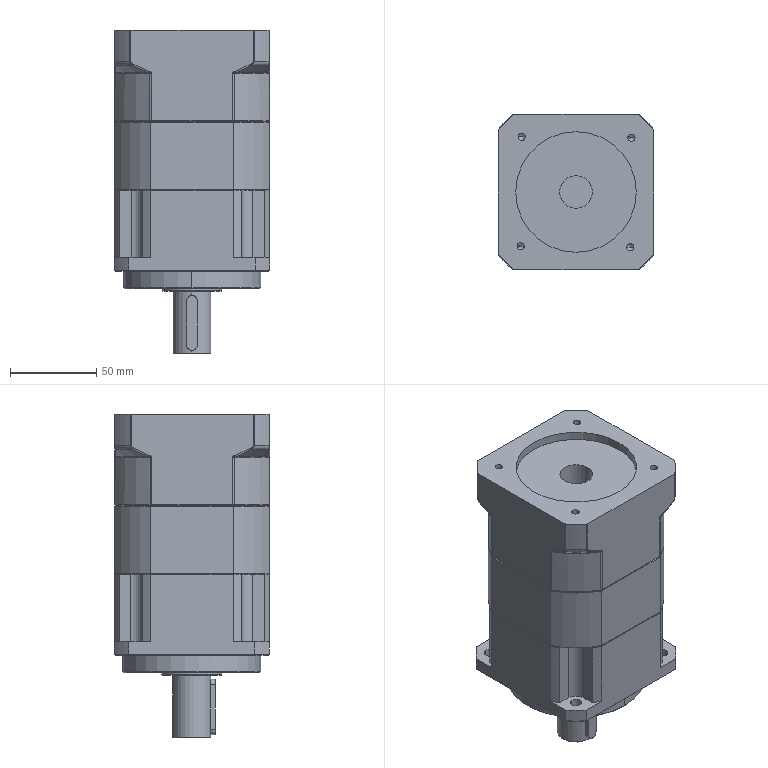Part | SolidWorks | features BaseBody 2 | 2 solids | 272 faces | box 90.02 x 90.185 x 188 mm | volume 989855 mm3 | cylinder 99 | plane 71 | cone 62 | spline 40 | commonest cylinder face diameters 6.6 x16 102 x16 2 x8 4 x8 4.2 x8 13 x4